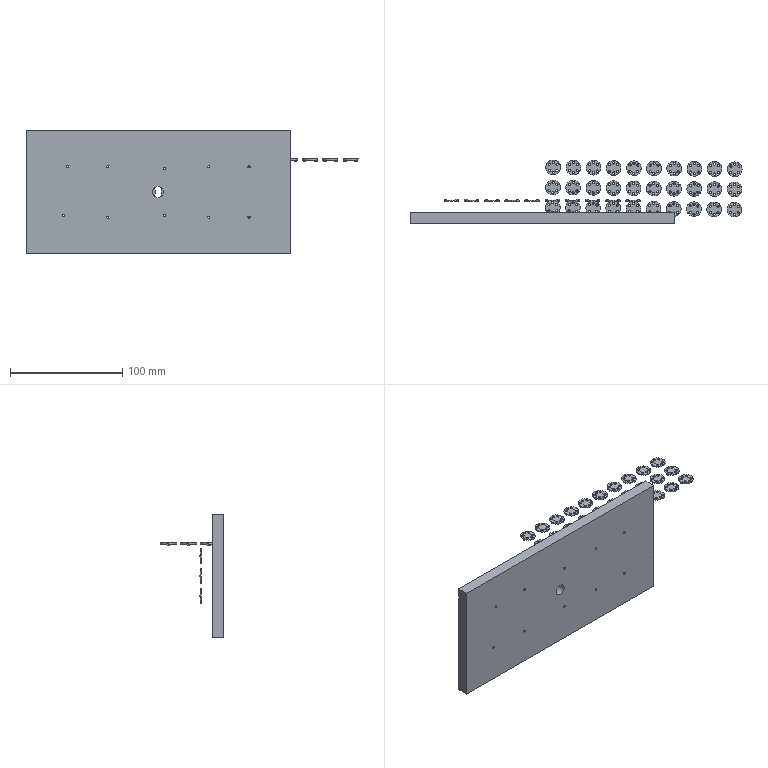Part | 61 solids | 1881 faces | box 296.27 x 56.878 x 110 mm | volume 265264 mm3 | plane 1208 | cylinder 673 | commonest cylinder face diameters 2 x372 1 x240 13 x60 10 x1